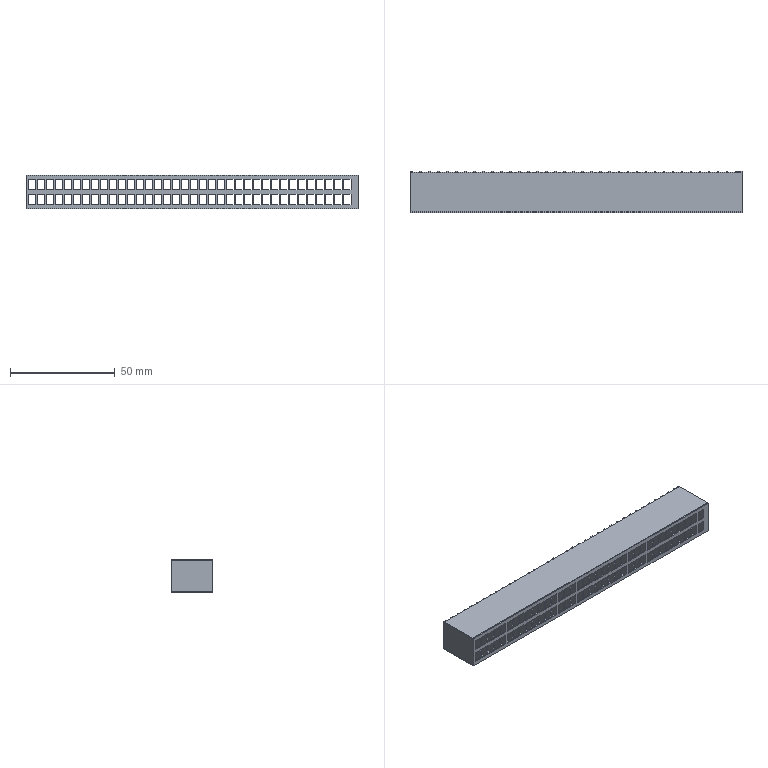Part | SolidWorks | features ICE 3, Extrusion 1, MirrorPattern 1 | 3 solids | 530 faces | box 158.568 x 20 x 16 mm | volume 13194 mm3 | plane 530